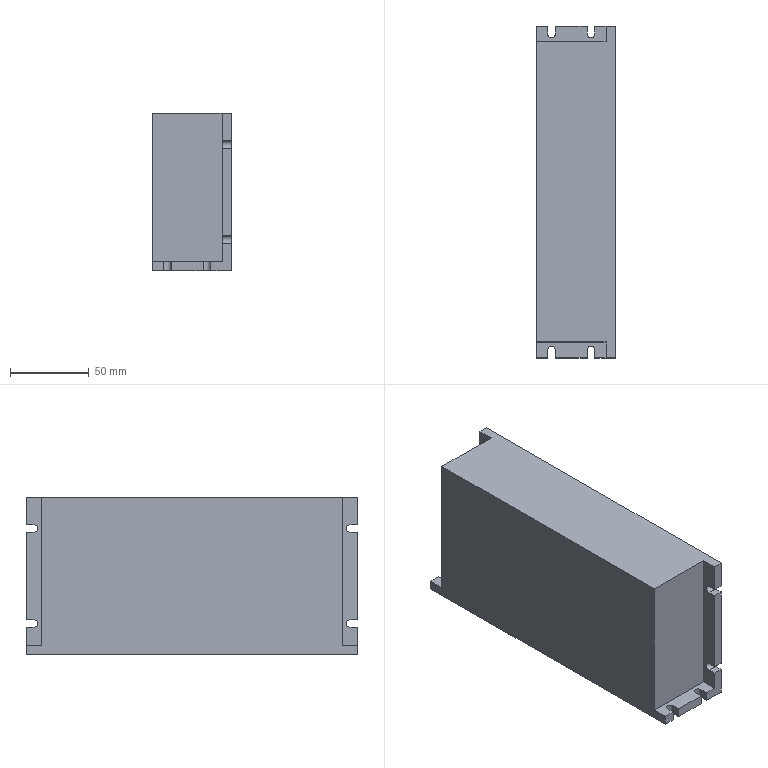Part | SolidWorks | features HoleWzd 2, Extrusion 1, ICE 1 | 1 solid | 44 faces | box 50 x 210 x 100 mm | volume 965694 mm3 | plane 36 | cylinder 8 | commonest cylinder face diameters 4.8 x8
STEP:
#1=CARTESIAN_POINT('',(-17.9,105.,6.));
#2=VERTEX_POINT('',#1);
#3=CARTESIAN_POINT('',(-25.,105.,6.));
#4=VERTEX_POINT('',#3);
#5=CARTESIAN_POINT('',(-25.,105.,6.));
#6=DIRECTION('',(-1.,0.,0.));
#7=VECTOR('',#6,1000.);
#8=LINE('',#5,#7);
#9=EDGE_CURVE('',#2,#4,#8,.T.);
#10=ORIENTED_EDGE('',*,*,#9,.F.);
#11=CARTESIAN_POINT('',(-17.9,105.,0.));
#12=VERTEX_POINT('',#11);
#13=CARTESIAN_POINT('',(-17.9,105.,100.));
#14=DIRECTION('',(0.,0.,-1.));
#15=VECTOR('',#14,1000.);
#16=LINE('',#13,#15);
#17=EDGE_CURVE('',#2,#12,#16,.T.);
#18=ORIENTED_EDGE('',*,*,#17,.T.);
#19=CARTESIAN_POINT('',(-25.,105.,0.));
#20=VERTEX_POINT('',#19);
#21=CARTESIAN_POINT('',(-25.,105.,0.));
#22=DIRECTION('',(-1.,0.,0.));
#23=VECTOR('',#22,1000.);
#24=LINE('',#21,#23);
#25=EDGE_CURVE('',#12,#20,#24,.T.);
#26=ORIENTED_EDGE('',*,*,#25,.T.);
#27=CARTESIAN_POINT('',(-25.,105.,100.));
#28=DIRECTION('',(0.,0.,-1.));
#29=VECTOR('',#28,1000.);
#30=LINE('',#27,#29);
#31=EDGE_CURVE('',#4,#20,#30,.T.);
#32=ORIENTED_EDGE('',*,*,#31,.F.);
#33=EDGE_LOOP('',(#10,#18,#26,#32));
#34=FACE_OUTER_BOUND('',#33,.T.);
#35=CARTESIAN_POINT('',(-25.,105.,100.));
#36=DIRECTION('',(0.,-1.,0.));
#37=DIRECTION('',(0.,0.,-1.));
#38=AXIS2_PLACEMENT_3D('',#35,#36,#37);
#39=PLANE('',#38);
#40=ADVANCED_FACE('',(#34),#39,.F.);
#41=CARTESIAN_POINT('',(7.1,105.,0.));
#42=VERTEX_POINT('',#41);
#43=CARTESIAN_POINT('',(-13.1,105.,0.));
#44=VERTEX_POINT('',#43);
#45=CARTESIAN_POINT('',(-25.,105.,0.));
#46=DIRECTION('',(-1.,0.,0.));
#47=VECTOR('',#46,1000.);
#48=LINE('',#45,#47);
#49=EDGE_CURVE('',#42,#44,#48,.T.);
#50=ORIENTED_EDGE('',*,*,#49,.T.);
#51=CARTESIAN_POINT('',(-13.1,105.,6.));
#52=VERTEX_POINT('',#51);
#53=CARTESIAN_POINT('',(-13.1,105.,100.));
#54=DIRECTION('',(0.,0.,1.));
#55=VECTOR('',#54,1000.);
#56=LINE('',#53,#55);
#57=EDGE_CURVE('',#44,#52,#56,.T.);
#58=ORIENTED_EDGE('',*,*,#57,.T.);
#59=CARTESIAN_POINT('',(7.1,105.,6.));
#60=VERTEX_POINT('',#59);
#61=CARTESIAN_POINT('',(-25.,105.,6.));
#62=DIRECTION('',(-1.,0.,0.));
#63=VECTOR('',#62,1000.);
#64=LINE('',#61,#63);
#65=EDGE_CURVE('',#60,#52,#64,.T.);
#66=ORIENTED_EDGE('',*,*,#65,.F.);
#67=CARTESIAN_POINT('',(7.1,105.,100.));
#68=DIRECTION('',(0.,0.,-1.));
#69=VECTOR('',#68,1000.);
#70=LINE('',#67,#69);
#71=EDGE_CURVE('',#60,#42,#70,.T.);
#72=ORIENTED_EDGE('',*,*,#71,.T.);
#73=EDGE_LOOP('',(#50,#58,#66,#72));
#74=FACE_OUTER_BOUND('',#73,.T.);
#75=CARTESIAN_POINT('',(-25.,105.,100.));
#76=DIRECTION('',(0.,-1.,0.));
#77=DIRECTION('',(0.,0.,-1.));
#78=AXIS2_PLACEMENT_3D('',#75,#76,#77);
#79=PLANE('',#78);
#80=ADVANCED_FACE('',(#74),#79,.F.);
#81=CARTESIAN_POINT('',(-13.1,-105.,0.));
#82=VERTEX_POINT('',#81);
#83=CARTESIAN_POINT('',(7.1,-105.,0.));
#84=VERTEX_POINT('',#83);
#85=CARTESIAN_POINT('',(-25.,-105.,0.));
#86=DIRECTION('',(1.,0.,0.));
#87=VECTOR('',#86,1000.);
#88=LINE('',#85,#87);
#89=EDGE_CURVE('',#82,#84,#88,.T.);
#90=ORIENTED_EDGE('',*,*,#89,.T.);
#91=CARTESIAN_POINT('',(7.1,-105.,6.));
#92=VERTEX_POINT('',#91);
#93=CARTESIAN_POINT('',(7.1,-105.,100.));
#94=DIRECTION('',(0.,0.,1.));
#95=VECTOR('',#94,1000.);
#96=LINE('',#93,#95);
#97=EDGE_CURVE('',#84,#92,#96,.T.);
#98=ORIENTED_EDGE('',*,*,#97,.T.);
#99=CARTESIAN_POINT('',(-13.1,-105.,6.));
#100=VERTEX_POINT('',#99);
#101=CARTESIAN_POINT('',(-25.,-105.,6.));
#102=DIRECTION('',(1.,0.,0.));
#103=VECTOR('',#102,1000.);
#104=LINE('',#101,#103);
#105=EDGE_CURVE('',#100,#92,#104,.T.);
#106=ORIENTED_EDGE('',*,*,#105,.F.);
#107=CARTESIAN_POINT('',(-13.1,-105.,100.));
#108=DIRECTION('',(0.,0.,-1.));
#109=VECTOR('',#108,1000.);
#110=LINE('',#107,#109);
#111=EDGE_CURVE('',#100,#82,#110,.T.);
#112=ORIENTED_EDGE('',*,*,#111,.T.);
#113=EDGE_LOOP('',(#90,#98,#106,#112));
#114=FACE_OUTER_BOUND('',#113,.T.);
#115=CARTESIAN_POINT('',(-25.,-105.,100.));
#116=DIRECTION('',(0.,1.,0.));
#117=DIRECTION('',(0.,0.,1.));
#118=AXIS2_PLACEMENT_3D('',#115,#116,#117);
#119=PLANE('',#118);
#120=ADVANCED_FACE('',(#114),#119,.F.);
#121=CARTESIAN_POINT('',(-25.,-105.,0.));
#122=VERTEX_POINT('',#121);
#123=CARTESIAN_POINT('',(-17.9,-105.,0.));
#124=VERTEX_POINT('',#123);
#125=CARTESIAN_POINT('',(-25.,-105.,0.));
#126=DIRECTION('',(1.,0.,0.));
#127=VECTOR('',#126,1000.);
#128=LINE('',#125,#127);
#129=EDGE_CURVE('',#122,#124,#128,.T.);
#130=ORIENTED_EDGE('',*,*,#129,.T.);
#131=CARTESIAN_POINT('',(-17.9,-105.,6.));
#132=VERTEX_POINT('',#131);
#133=CARTESIAN_POINT('',(-17.9,-105.,100.));
#134=DIRECTION('',(0.,0.,1.));
#135=VECTOR('',#134,1000.);
#136=LINE('',#133,#135);
#137=EDGE_CURVE('',#124,#132,#136,.T.);
#138=ORIENTED_EDGE('',*,*,#137,.T.);
#139=CARTESIAN_POINT('',(-25.,-105.,6.));
#140=VERTEX_POINT('',#139);
#141=CARTESIAN_POINT('',(-25.,-105.,6.));
#142=DIRECTION('',(1.,0.,0.));
#143=VECTOR('',#142,1000.);
#144=LINE('',#141,#143);
#145=EDGE_CURVE('',#140,#132,#144,.T.);
#146=ORIENTED_EDGE('',*,*,#145,.F.);
#147=CARTESIAN_POINT('',(-25.,-105.,100.));
#148=DIRECTION('',(0.,0.,-1.));
#149=VECTOR('',#148,1000.);
#150=LINE('',#147,#149);
#151=EDGE_CURVE('',#140,#122,#150,.T.);
#152=ORIENTED_EDGE('',*,*,#151,.T.);
#153=EDGE_LOOP('',(#130,#138,#146,#152));
#154=FACE_OUTER_BOUND('',#153,.T.);
#155=CARTESIAN_POINT('',(-25.,-105.,100.));
#156=DIRECTION('',(0.,1.,0.));
#157=DIRECTION('',(0.,0.,1.));
#158=AXIS2_PLACEMENT_3D('',#155,#156,#157);
#159=PLANE('',#158);
#160=ADVANCED_FACE('',(#154),#159,.F.);
#161=CARTESIAN_POINT('',(25.,105.,100.));
#162=VERTEX_POINT('',#161);
#163=CARTESIAN_POINT('',(25.,105.,82.4));
#164=VERTEX_POINT('',#163);
#165=CARTESIAN_POINT('',(25.,105.,100.));
#166=DIRECTION('',(0.,0.,-1.));
#167=VECTOR('',#166,1000.);
#168=LINE('',#165,#167);
#169=EDGE_CURVE('',#162,#164,#168,.T.);
#170=ORIENTED_EDGE('',*,*,#169,.T.);
#171=CARTESIAN_POINT('',(19.,105.,82.4));
#172=VERTEX_POINT('',#171);
#173=CARTESIAN_POINT('',(-25.,105.,82.4));
#174=DIRECTION('',(-1.,0.,0.));
#175=VECTOR('',#174,1000.);
#176=LINE('',#173,#175);
#177=EDGE_CURVE('',#164,#172,#176,.T.);
#178=ORIENTED_EDGE('',*,*,#177,.T.);
#179=CARTESIAN_POINT('',(19.,105.,100.));
#180=VERTEX_POINT('',#179);
#181=CARTESIAN_POINT('',(19.,105.,-45.122));
#182=DIRECTION('',(0.,0.,1.));
#183=VECTOR('',#182,1000.);
#184=LINE('',#181,#183);
#185=EDGE_CURVE('',#172,#180,#184,.T.);
#186=ORIENTED_EDGE('',*,*,#185,.T.);
#187=CARTESIAN_POINT('',(-25.,105.,100.));
#188=DIRECTION('',(-1.,0.,0.));
#189=VECTOR('',#188,1000.);
#190=LINE('',#187,#189);
#191=EDGE_CURVE('',#162,#180,#190,.T.);
#192=ORIENTED_EDGE('',*,*,#191,.F.);
#193=EDGE_LOOP('',(#170,#178,#186,#192));
#194=FACE_OUTER_BOUND('',#193,.T.);
#195=CARTESIAN_POINT('',(-25.,105.,100.));
#196=DIRECTION('',(0.,-1.,0.));
#197=DIRECTION('',(0.,0.,-1.));
#198=AXIS2_PLACEMENT_3D('',#195,#196,#197);
#199=PLANE('',#198);
#200=ADVANCED_FACE('',(#194),#199,.F.);
#201=CARTESIAN_POINT('',(19.,105.,22.4));
#202=VERTEX_POINT('',#201);
#203=CARTESIAN_POINT('',(19.,105.,77.6));
#204=VERTEX_POINT('',#203);
#205=CARTESIAN_POINT('',(19.,105.,-45.122));
#206=DIRECTION('',(0.,0.,1.));
#207=VECTOR('',#206,1000.);
#208=LINE('',#205,#207);
#209=EDGE_CURVE('',#202,#204,#208,.T.);
#210=ORIENTED_EDGE('',*,*,#209,.T.);
#211=CARTESIAN_POINT('',(25.,105.,77.6));
#212=VERTEX_POINT('',#211);
#213=CARTESIAN_POINT('',(-25.,105.,77.6));
#214=DIRECTION('',(1.,0.,0.));
#215=VECTOR('',#214,1000.);
#216=LINE('',#213,#215);
#217=EDGE_CURVE('',#204,#212,#216,.T.);
#218=ORIENTED_EDGE('',*,*,#217,.T.);
#219=CARTESIAN_POINT('',(25.,105.,22.4));
#220=VERTEX_POINT('',#219);
#221=CARTESIAN_POINT('',(25.,105.,100.));
#222=DIRECTION('',(0.,0.,-1.));
#223=VECTOR('',#222,1000.);
#224=LINE('',#221,#223);
#225=EDGE_CURVE('',#212,#220,#224,.T.);
#226=ORIENTED_EDGE('',*,*,#225,.T.);
#227=CARTESIAN_POINT('',(-25.,105.,22.4));
#228=DIRECTION('',(-1.,0.,0.));
#229=VECTOR('',#228,1000.);
#230=LINE('',#227,#229);
#231=EDGE_CURVE('',#220,#202,#230,.T.);
#232=ORIENTED_EDGE('',*,*,#231,.T.);
#233=EDGE_LOOP('',(#210,#218,#226,#232));
#234=FACE_OUTER_BOUND('',#233,.T.);
#235=CARTESIAN_POINT('',(-25.,105.,100.));
#236=DIRECTION('',(0.,-1.,0.));
#237=DIRECTION('',(0.,0.,-1.));
#238=AXIS2_PLACEMENT_3D('',#235,#236,#237);
#239=PLANE('',#238);
#240=ADVANCED_FACE('',(#234),#239,.F.);
#241=CARTESIAN_POINT('',(19.,-105.,22.4));
#242=VERTEX_POINT('',#241);
#243=CARTESIAN_POINT('',(19.,-105.,77.6));
#244=VERTEX_POINT('',#243);
#245=CARTESIAN_POINT('',(19.,-105.,-45.122));
#246=DIRECTION('',(0.,0.,1.));
#247=VECTOR('',#246,1000.);
#248=LINE('',#245,#247);
#249=EDGE_CURVE('',#242,#244,#248,.T.);
#250=ORIENTED_EDGE('',*,*,#249,.F.);
#251=CARTESIAN_POINT('',(25.,-105.,22.4));
#252=VERTEX_POINT('',#251);
#253=CARTESIAN_POINT('',(-25.,-105.,22.4));
#254=DIRECTION('',(1.,0.,0.));
#255=VECTOR('',#254,1000.);
#256=LINE('',#253,#255);
#257=EDGE_CURVE('',#242,#252,#256,.T.);
#258=ORIENTED_EDGE('',*,*,#257,.T.);
#259=CARTESIAN_POINT('',(25.,-105.,77.6));
#260=VERTEX_POINT('',#259);
#261=CARTESIAN_POINT('',(25.,-105.,100.));
#262=DIRECTION('',(0.,0.,-1.));
#263=VECTOR('',#262,1000.);
#264=LINE('',#261,#263);
#265=EDGE_CURVE('',#260,#252,#264,.T.);
#266=ORIENTED_EDGE('',*,*,#265,.F.);
#267=CARTESIAN_POINT('',(-25.,-105.,77.6));
#268=DIRECTION('',(-1.,0.,0.));
#269=VECTOR('',#268,1000.);
#270=LINE('',#267,#269);
#271=EDGE_CURVE('',#260,#244,#270,.T.);
#272=ORIENTED_EDGE('',*,*,#271,.T.);
#273=EDGE_LOOP('',(#250,#258,#266,#272));
#274=FACE_OUTER_BOUND('',#273,.T.);
#275=CARTESIAN_POINT('',(-25.,-105.,100.));
#276=DIRECTION('',(0.,1.,0.));
#277=DIRECTION('',(0.,0.,1.));
#278=AXIS2_PLACEMENT_3D('',#275,#276,#277);
#279=PLANE('',#278);
#280=ADVANCED_FACE('',(#274),#279,.F.);
#281=CARTESIAN_POINT('',(19.,-105.,82.4));
#282=VERTEX_POINT('',#281);
#283=CARTESIAN_POINT('',(19.,-105.,100.));
#284=VERTEX_POINT('',#283);
#285=CARTESIAN_POINT('',(19.,-105.,-45.122));
#286=DIRECTION('',(0.,0.,1.));
#287=VECTOR('',#286,1000.);
#288=LINE('',#285,#287);
#289=EDGE_CURVE('',#282,#284,#288,.T.);
#290=ORIENTED_EDGE('',*,*,#289,.F.);
#291=CARTESIAN_POINT('',(25.,-105.,82.4));
#292=VERTEX_POINT('',#291);
#293=CARTESIAN_POINT('',(-25.,-105.,82.4));
#294=DIRECTION('',(1.,0.,0.));
#295=VECTOR('',#294,1000.);
#296=LINE('',#293,#295);
#297=EDGE_CURVE('',#282,#292,#296,.T.);
#298=ORIENTED_EDGE('',*,*,#297,.T.);
#299=CARTESIAN_POINT('',(25.,-105.,100.));
#300=VERTEX_POINT('',#299);
#301=CARTESIAN_POINT('',(25.,-105.,100.));
#302=DIRECTION('',(0.,0.,-1.));
#303=VECTOR('',#302,1000.);
#304=LINE('',#301,#303);
#305=EDGE_CURVE('',#300,#292,#304,.T.);
#306=ORIENTED_EDGE('',*,*,#305,.F.);
#307=CARTESIAN_POINT('',(-25.,-105.,100.));
#308=DIRECTION('',(1.,0.,0.));
#309=VECTOR('',#308,1000.);
#310=LINE('',#307,#309);
#311=EDGE_CURVE('',#284,#300,#310,.T.);
#312=ORIENTED_EDGE('',*,*,#311,.F.);
#313=EDGE_LOOP('',(#290,#298,#306,#312));
#314=FACE_OUTER_BOUND('',#313,.T.);
#315=CARTESIAN_POINT('',(-25.,-105.,100.));
#316=DIRECTION('',(0.,1.,0.));
#317=DIRECTION('',(0.,0.,1.));
#318=AXIS2_PLACEMENT_3D('',#315,#316,#317);
#319=PLANE('',#318);
#320=ADVANCED_FACE('',(#314),#319,.F.);
#321=CARTESIAN_POINT('',(25.,100.,82.4));
#322=VERTEX_POINT('',#321);
#323=CARTESIAN_POINT('',(25.,100.,77.6));
#324=VERTEX_POINT('',#323);
#325=CARTESIAN_POINT('',(25.,100.,80.));
#326=DIRECTION('',(1.,0.,0.));
#327=DIRECTION('',(0.,0.,-1.));
#328=AXIS2_PLACEMENT_3D('',#325,#326,#327);
#329=CIRCLE('',#328,2.4);
#330=EDGE_CURVE('',#322,#324,#329,.T.);
#331=ORIENTED_EDGE('',*,*,#330,.F.);
#332=CARTESIAN_POINT('',(25.,100.,82.4));
#333=DIRECTION('',(0.,1.,0.));
#334=VECTOR('',#333,1000.);
#335=LINE('',#332,#334);
#336=EDGE_CURVE('',#322,#164,#335,.T.);
#337=ORIENTED_EDGE('',*,*,#336,.T.);
#338=ORIENTED_EDGE('',*,*,#169,.F.);
#339=CARTESIAN_POINT('',(25.,-105.,100.));
#340=DIRECTION('',(0.,1.,0.));
#341=VECTOR('',#340,1000.);
#342=LINE('',#339,#341);
#343=EDGE_CURVE('',#300,#162,#342,.T.);
#344=ORIENTED_EDGE('',*,*,#343,.F.);
#345=ORIENTED_EDGE('',*,*,#305,.T.);
#346=CARTESIAN_POINT('',(25.,-100.,82.4));
#347=VERTEX_POINT('',#346);
#348=CARTESIAN_POINT('',(25.,-110.,82.4));
#349=DIRECTION('',(0.,1.,0.));
#350=VECTOR('',#349,1000.);
#351=LINE('',#348,#350);
#352=EDGE_CURVE('',#292,#347,#351,.T.);
#353=ORIENTED_EDGE('',*,*,#352,.T.);
#354=CARTESIAN_POINT('',(25.,-100.,77.6));
#355=VERTEX_POINT('',#354);
#356=CARTESIAN_POINT('',(25.,-100.,80.));
#357=DIRECTION('',(1.,0.,0.));
#358=DIRECTION('',(0.,0.,-1.));
#359=AXIS2_PLACEMENT_3D('',#356,#357,#358);
#360=CIRCLE('',#359,2.4);
#361=EDGE_CURVE('',#355,#347,#360,.T.);
#362=ORIENTED_EDGE('',*,*,#361,.F.);
#363=CARTESIAN_POINT('',(25.,-110.,77.6));
#364=DIRECTION('',(0.,1.,0.));
#365=VECTOR('',#364,1000.);
#366=LINE('',#363,#365);
#367=EDGE_CURVE('',#260,#355,#366,.T.);
#368=ORIENTED_EDGE('',*,*,#367,.F.);
#369=ORIENTED_EDGE('',*,*,#265,.T.);
#370=CARTESIAN_POINT('',(25.,-100.,22.4));
#371=VERTEX_POINT('',#370);
#372=CARTESIAN_POINT('',(25.,-110.,22.4));
#373=DIRECTION('',(0.,1.,0.));
#374=VECTOR('',#373,1000.);
#375=LINE('',#372,#374);
#376=EDGE_CURVE('',#252,#371,#375,.T.);
#377=ORIENTED_EDGE('',*,*,#376,.T.);
#378=CARTESIAN_POINT('',(25.,-100.,17.6));
#379=VERTEX_POINT('',#378);
#380=CARTESIAN_POINT('',(25.,-100.,20.));
#381=DIRECTION('',(1.,0.,0.));
#382=DIRECTION('',(0.,0.,-1.));
#383=AXIS2_PLACEMENT_3D('',#380,#381,#382);
#384=CIRCLE('',#383,2.4);
#385=EDGE_CURVE('',#379,#371,#384,.T.);
#386=ORIENTED_EDGE('',*,*,#385,.F.);
#387=CARTESIAN_POINT('',(25.,-105.,17.6));
#388=VERTEX_POINT('',#387);
#389=CARTESIAN_POINT('',(25.,-110.,17.6));
#390=DIRECTION('',(0.,1.,0.));
#391=VECTOR('',#390,1000.);
#392=LINE('',#389,#391);
#393=EDGE_CURVE('',#388,#379,#392,.T.);
#394=ORIENTED_EDGE('',*,*,#393,.F.);
#395=CARTESIAN_POINT('',(25.,-105.,0.));
#396=VERTEX_POINT('',#395);
#397=CARTESIAN_POINT('',(25.,-105.,100.));
#398=DIRECTION('',(0.,0.,-1.));
#399=VECTOR('',#398,1000.);
#400=LINE('',#397,#399);
#401=EDGE_CURVE('',#388,#396,#400,.T.);
#402=ORIENTED_EDGE('',*,*,#401,.T.);
#403=CARTESIAN_POINT('',(25.,105.,0.));
#404=VERTEX_POINT('',#403);
#405=CARTESIAN_POINT('',(25.,-105.,0.));
#406=DIRECTION('',(0.,1.,0.));
#407=VECTOR('',#406,1000.);
#408=LINE('',#405,#407);
#409=EDGE_CURVE('',#396,#404,#408,.T.);
#410=ORIENTED_EDGE('',*,*,#409,.T.);
#411=CARTESIAN_POINT('',(25.,105.,17.6));
#412=VERTEX_POINT('',#411);
#413=CARTESIAN_POINT('',(25.,105.,100.));
#414=DIRECTION('',(0.,0.,-1.));
#415=VECTOR('',#414,1000.);
#416=LINE('',#413,#415);
#417=EDGE_CURVE('',#412,#404,#416,.T.);
#418=ORIENTED_EDGE('',*,*,#417,.F.);
#419=CARTESIAN_POINT('',(25.,100.,17.6));
#420=VERTEX_POINT('',#419);
#421=CARTESIAN_POINT('',(25.,100.,17.6));
#422=DIRECTION('',(0.,1.,0.));
#423=VECTOR('',#422,1000.);
#424=LINE('',#421,#423);
#425=EDGE_CURVE('',#420,#412,#424,.T.);
#426=ORIENTED_EDGE('',*,*,#425,.F.);
#427=CARTESIAN_POINT('',(25.,100.,22.4));
#428=VERTEX_POINT('',#427);
#429=CARTESIAN_POINT('',(25.,100.,20.));
#430=DIRECTION('',(1.,0.,0.));
#431=DIRECTION('',(0.,0.,-1.));
#432=AXIS2_PLACEMENT_3D('',#429,#430,#431);
#433=CIRCLE('',#432,2.4);
#434=EDGE_CURVE('',#428,#420,#433,.T.);
#435=ORIENTED_EDGE('',*,*,#434,.F.);
#436=CARTESIAN_POINT('',(25.,100.,22.4));
#437=DIRECTION('',(0.,1.,0.));
#438=VECTOR('',#437,1000.);
#439=LINE('',#436,#438);
#440=EDGE_CURVE('',#428,#220,#439,.T.);
#441=ORIENTED_EDGE('',*,*,#440,.T.);
#442=ORIENTED_EDGE('',*,*,#225,.F.);
#443=CARTESIAN_POINT('',(25.,100.,77.6));
#444=DIRECTION('',(0.,1.,0.));
#445=VECTOR('',#444,1000.);
#446=LINE('',#443,#445);
#447=EDGE_CURVE('',#324,#212,#446,.T.);
#448=ORIENTED_EDGE('',*,*,#447,.F.);
#449=EDGE_LOOP('',(#331,#337,#338,#344,#345,#353,#362,#368,#369,#377,#386,#394,#402,#410,#418,#426,#435,#441,#442,#448));
#450=FACE_OUTER_BOUND('',#449,.T.);
#451=CARTESIAN_POINT('',(25.,-105.,100.));
#452=DIRECTION('',(-1.,0.,0.));
#453=DIRECTION('',(0.,0.,1.));
#454=AXIS2_PLACEMENT_3D('',#451,#452,#453);
#455=PLANE('',#454);
#456=ADVANCED_FACE('',(#450),#455,.F.);
#457=CARTESIAN_POINT('',(11.9,105.,0.));
#458=VERTEX_POINT('',#457);
#459=CARTESIAN_POINT('',(-25.,105.,0.));
#460=DIRECTION('',(-1.,0.,0.));
#461=VECTOR('',#460,1000.);
#462=LINE('',#459,#461);
#463=EDGE_CURVE('',#404,#458,#462,.T.);
#464=ORIENTED_EDGE('',*,*,#463,.T.);
#465=CARTESIAN_POINT('',(11.9,105.,6.));
#466=VERTEX_POINT('',#465);
#467=CARTESIAN_POINT('',(11.9,105.,100.));
#468=DIRECTION('',(0.,0.,1.));
#469=VECTOR('',#468,1000.);
#470=LINE('',#467,#469);
#471=EDGE_CURVE('',#458,#466,#470,.T.);
#472=ORIENTED_EDGE('',*,*,#471,.T.);
#473=CARTESIAN_POINT('',(19.,105.,6.));
#474=VERTEX_POINT('',#473);
#475=CARTESIAN_POINT('',(-25.,105.,6.));
#476=DIRECTION('',(-1.,0.,0.));
#477=VECTOR('',#476,1000.);
#478=LINE('',#475,#477);
#479=EDGE_CURVE('',#474,#466,#478,.T.);
#480=ORIENTED_EDGE('',*,*,#479,.F.);
#481=CARTESIAN_POINT('',(19.,105.,17.6));
#482=VERTEX_POINT('',#481);
#483=CARTESIAN_POINT('',(19.,105.,-45.122));
#484=DIRECTION('',(0.,0.,1.));
#485=VECTOR('',#484,1000.);
#486=LINE('',#483,#485);
#487=EDGE_CURVE('',#474,#482,#486,.T.);
#488=ORIENTED_EDGE('',*,*,#487,.T.);
#489=CARTESIAN_POINT('',(-25.,105.,17.6));
#490=DIRECTION('',(1.,0.,0.));
#491=VECTOR('',#490,1000.);
#492=LINE('',#489,#491);
#493=EDGE_CURVE('',#482,#412,#492,.T.);
#494=ORIENTED_EDGE('',*,*,#493,.T.);
#495=ORIENTED_EDGE('',*,*,#417,.T.);
#496=EDGE_LOOP('',(#464,#472,#480,#488,#494,#495));
#497=FACE_OUTER_BOUND('',#496,.T.);
#498=CARTESIAN_POINT('',(-25.,105.,100.));
#499=DIRECTION('',(0.,-1.,0.));
#500=DIRECTION('',(0.,0.,-1.));
#501=AXIS2_PLACEMENT_3D('',#498,#499,#500);
#502=PLANE('',#501);
#503=ADVANCED_FACE('',(#497),#502,.F.);
#504=CARTESIAN_POINT('',(-25.,95.,6.));
#505=VERTEX_POINT('',#504);
#506=CARTESIAN_POINT('',(-25.,95.,100.));
#507=VERTEX_POINT('',#506);
#508=CARTESIAN_POINT('',(-25.,95.,-45.122));
#509=DIRECTION('',(0.,0.,1.));
#510=VECTOR('',#509,1000.);
#511=LINE('',#508,#510);
#512=EDGE_CURVE('',#505,#507,#511,.T.);
#513=ORIENTED_EDGE('',*,*,#512,.F.);
#514=CARTESIAN_POINT('',(-25.,105.,6.));
#515=DIRECTION('',(0.,-1.,0.));
#516=VECTOR('',#515,1000.);
#517=LINE('',#514,#516);
#518=EDGE_CURVE('',#4,#505,#517,.T.);
#519=ORIENTED_EDGE('',*,*,#518,.F.);
#520=ORIENTED_EDGE('',*,*,#31,.T.);
#521=CARTESIAN_POINT('',(-25.,-105.,0.));
#522=DIRECTION('',(0.,-1.,0.));
#523=VECTOR('',#522,1000.);
#524=LINE('',#521,#523);
#525=EDGE_CURVE('',#20,#122,#524,.T.);
#526=ORIENTED_EDGE('',*,*,#525,.T.);
#527=ORIENTED_EDGE('',*,*,#151,.F.);
#528=CARTESIAN_POINT('',(-25.,-95.,6.));
#529=VERTEX_POINT('',#528);
#530=CARTESIAN_POINT('',(-25.,-105.,6.));
#531=DIRECTION('',(0.,-1.,0.));
#532=VECTOR('',#531,1000.);
#533=LINE('',#530,#532);
#534=EDGE_CURVE('',#529,#140,#533,.T.);
#535=ORIENTED_EDGE('',*,*,#534,.F.);
#536=CARTESIAN_POINT('',(-25.,-95.,100.));
#537=VERTEX_POINT('',#536);
#538=CARTESIAN_POINT('',(-25.,-95.,-45.122));
#539=DIRECTION('',(0.,0.,1.));
#540=VECTOR('',#539,1000.);
#541=LINE('',#538,#540);
#542=EDGE_CURVE('',#529,#537,#541,.T.);
#543=ORIENTED_EDGE('',*,*,#542,.T.);
#544=CARTESIAN_POINT('',(-25.,-105.,100.));
#545=DIRECTION('',(0.,-1.,0.));
#546=VECTOR('',#545,1000.);
#547=LINE('',#544,#546);
#548=EDGE_CURVE('',#507,#537,#547,.T.);
#549=ORIENTED_EDGE('',*,*,#548,.F.);
#550=EDGE_LOOP('',(#513,#519,#520,#526,#527,#535,#543,#549));
#551=FACE_OUTER_BOUND('',#550,.T.);
#552=CARTESIAN_POINT('',(-25.,-105.,100.));
#553=DIRECTION('',(1.,0.,0.));
#554=DIRECTION('',(0.,0.,-1.));
#555=AXIS2_PLACEMENT_3D('',#552,#553,#554);
#556=PLANE('',#555);
#557=ADVANCED_FACE('',(#551),#556,.F.);
#558=CARTESIAN_POINT('',(11.9,-105.,6.));
#559=VERTEX_POINT('',#558);
#560=CARTESIAN_POINT('',(19.,-105.,6.));
#561=VERTEX_POINT('',#560);
#562=CARTESIAN_POINT('',(-25.,-105.,6.));
#563=DIRECTION('',(1.,0.,0.));
#564=VECTOR('',#563,1000.);
#565=LINE('',#562,#564);
#566=EDGE_CURVE('',#559,#561,#565,.T.);
#567=ORIENTED_EDGE('',*,*,#566,.F.);
#568=CARTESIAN_POINT('',(11.9,-105.,0.));
#569=VERTEX_POINT('',#568);
#570=CARTESIAN_POINT('',(11.9,-105.,100.));
#571=DIRECTION('',(0.,0.,-1.));
#572=VECTOR('',#571,1000.);
#573=LINE('',#570,#572);
#574=EDGE_CURVE('',#559,#569,#573,.T.);
#575=ORIENTED_EDGE('',*,*,#574,.T.);
#576=CARTESIAN_POINT('',(-25.,-105.,0.));
#577=DIRECTION('',(1.,0.,0.));
#578=VECTOR('',#577,1000.);
#579=LINE('',#576,#578);
#580=EDGE_CURVE('',#569,#396,#579,.T.);
#581=ORIENTED_EDGE('',*,*,#580,.T.);
#582=ORIENTED_EDGE('',*,*,#401,.F.);
#583=CARTESIAN_POINT('',(19.,-105.,17.6));
#584=VERTEX_POINT('',#583);
#585=CARTESIAN_POINT('',(-25.,-105.,17.6));
#586=DIRECTION('',(-1.,0.,0.));
#587=VECTOR('',#586,1000.);
#588=LINE('',#585,#587);
#589=EDGE_CURVE('',#388,#584,#588,.T.);
#590=ORIENTED_EDGE('',*,*,#589,.T.);
#591=CARTESIAN_POINT('',(19.,-105.,-45.122));
#592=DIRECTION('',(0.,0.,1.));
#593=VECTOR('',#592,1000.);
#594=LINE('',#591,#593);
#595=EDGE_CURVE('',#561,#584,#594,.T.);
#596=ORIENTED_EDGE('',*,*,#595,.F.);
#597=EDGE_LOOP('',(#567,#575,#581,#582,#590,#596));
#598=FACE_OUTER_BOUND('',#597,.T.);
#599=CARTESIAN_POINT('',(-25.,-105.,100.));
#600=DIRECTION('',(0.,1.,0.));
#601=DIRECTION('',(0.,0.,1.));
#602=AXIS2_PLACEMENT_3D('',#599,#600,#601);
#603=PLANE('',#602);
#604=ADVANCED_FACE('',(#598),#603,.F.);
#605=CARTESIAN_POINT('',(19.,95.,100.));
#606=VERTEX_POINT('',#605);
#607=CARTESIAN_POINT('',(19.,105.,100.));
#608=DIRECTION('',(0.,1.,0.));
#609=VECTOR('',#608,1000.);
#610=LINE('',#607,#609);
#611=EDGE_CURVE('',#606,#180,#610,.T.);
#612=ORIENTED_EDGE('',*,*,#611,.F.);
#613=CARTESIAN_POINT('',(-25.,95.,100.));
#614=DIRECTION('',(1.,0.,0.));
#615=VECTOR('',#614,1000.);
#616=LINE('',#613,#615);
#617=EDGE_CURVE('',#507,#606,#616,.T.);
#618=ORIENTED_EDGE('',*,*,#617,.F.);
#619=ORIENTED_EDGE('',*,*,#548,.T.);
#620=CARTESIAN_POINT('',(19.,-95.,100.));
#621=VERTEX_POINT('',#620);
#622=CARTESIAN_POINT('',(-25.,-95.,100.));
#623=DIRECTION('',(-1.,0.,0.));
#624=VECTOR('',#623,1000.);
#625=LINE('',#622,#624);
#626=EDGE_CURVE('',#621,#537,#625,.T.);
#627=ORIENTED_EDGE('',*,*,#626,.F.);
#628=CARTESIAN_POINT('',(19.,-105.,100.));
#629=DIRECTION('',(0.,1.,0.));
#630=VECTOR('',#629,1000.);
#631=LINE('',#628,#630);
#632=EDGE_CURVE('',#284,#621,#631,.T.);
#633=ORIENTED_EDGE('',*,*,#632,.F.);
#634=ORIENTED_EDGE('',*,*,#311,.T.);
#635=ORIENTED_EDGE('',*,*,#343,.T.);
#636=ORIENTED_EDGE('',*,*,#191,.T.);
#637=EDGE_LOOP('',(#612,#618,#619,#627,#633,#634,#635,#636));
#638=FACE_OUTER_BOUND('',#637,.T.);
#639=CARTESIAN_POINT('',(0.,0.,100.));
#640=DIRECTION('',(0.,0.,-1.));
#641=DIRECTION('',(-1.,0.,0.));
#642=AXIS2_PLACEMENT_3D('',#639,#640,#641);
#643=PLANE('',#642);
#644=ADVANCED_FACE('',(#638),#643,.F.);
#645=CARTESIAN_POINT('',(-17.9,100.,0.));
#646=VERTEX_POINT('',#645);
#647=CARTESIAN_POINT('',(-17.9,100.,0.));
#648=DIRECTION('',(0.,1.,0.));
#649=VECTOR('',#648,1000.);
#650=LINE('',#647,#649);
#651=EDGE_CURVE('',#646,#12,#650,.T.);
#652=ORIENTED_EDGE('',*,*,#651,.F.);
#653=CARTESIAN_POINT('',(-13.1,100.,0.));
#654=VERTEX_POINT('',#653);
#655=CARTESIAN_POINT('',(-15.5,100.,0.));
#656=DIRECTION('',(0.,0.,1.));
#657=DIRECTION('',(1.,0.,0.));
#658=AXIS2_PLACEMENT_3D('',#655,#656,#657);
#659=CIRCLE('',#658,2.4);
#660=EDGE_CURVE('',#646,#654,#659,.T.);
#661=ORIENTED_EDGE('',*,*,#660,.T.);
#662=CARTESIAN_POINT('',(-13.1,100.,0.));
#663=DIRECTION('',(0.,1.,0.));
#664=VECTOR('',#663,1000.);
#665=LINE('',#662,#664);
#666=EDGE_CURVE('',#654,#44,#665,.T.);
#667=ORIENTED_EDGE('',*,*,#666,.T.);
#668=ORIENTED_EDGE('',*,*,#49,.F.);
#669=CARTESIAN_POINT('',(7.1,100.,0.));
#670=VERTEX_POINT('',#669);
#671=CARTESIAN_POINT('',(7.1,100.,0.));
#672=DIRECTION('',(0.,1.,0.));
#673=VECTOR('',#672,1000.);
#674=LINE('',#671,#673);
#675=EDGE_CURVE('',#670,#42,#674,.T.);
#676=ORIENTED_EDGE('',*,*,#675,.F.);
#677=CARTESIAN_POINT('',(11.9,100.,0.));
#678=VERTEX_POINT('',#677);
#679=CARTESIAN_POINT('',(9.5,100.,0.));
#680=DIRECTION('',(0.,0.,1.));
#681=DIRECTION('',(1.,0.,0.));
#682=AXIS2_PLACEMENT_3D('',#679,#680,#681);
#683=CIRCLE('',#682,2.4);
#684=EDGE_CURVE('',#670,#678,#683,.T.);
#685=ORIENTED_EDGE('',*,*,#684,.T.);
#686=CARTESIAN_POINT('',(11.9,100.,0.));
#687=DIRECTION('',(0.,1.,0.));
#688=VECTOR('',#687,1000.);
#689=LINE('',#686,#688);
#690=EDGE_CURVE('',#678,#458,#689,.T.);
#691=ORIENTED_EDGE('',*,*,#690,.T.);
#692=ORIENTED_EDGE('',*,*,#463,.F.);
#693=ORIENTED_EDGE('',*,*,#409,.F.);
#694=ORIENTED_EDGE('',*,*,#580,.F.);
#695=CARTESIAN_POINT('',(11.9,-100.,0.));
#696=VERTEX_POINT('',#695);
#697=CARTESIAN_POINT('',(11.9,0.,0.));
#698=DIRECTION('',(0.,-1.,0.));
#699=VECTOR('',#698,1000.);
#700=LINE('',#697,#699);
#701=EDGE_CURVE('',#696,#569,#700,.T.);
#702=ORIENTED_EDGE('',*,*,#701,.F.);
#703=CARTESIAN_POINT('',(7.1,-100.,0.));
#704=VERTEX_POINT('',#703);
#705=CARTESIAN_POINT('',(9.5,-100.,0.));
#706=DIRECTION('',(0.,0.,1.));
#707=DIRECTION('',(1.,0.,0.));
#708=AXIS2_PLACEMENT_3D('',#705,#706,#707);
#709=CIRCLE('',#708,2.4);
#710=EDGE_CURVE('',#696,#704,#709,.T.);
#711=ORIENTED_EDGE('',*,*,#710,.T.);
#712=CARTESIAN_POINT('',(7.1,0.,0.));
#713=DIRECTION('',(0.,1.,0.));
#714=VECTOR('',#713,1000.);
#715=LINE('',#712,#714);
#716=EDGE_CURVE('',#84,#704,#715,.T.);
#717=ORIENTED_EDGE('',*,*,#716,.F.);
#718=ORIENTED_EDGE('',*,*,#89,.F.);
#719=CARTESIAN_POINT('',(-13.1,-100.,0.));
#720=VERTEX_POINT('',#719);
#721=CARTESIAN_POINT('',(-13.1,-110.,0.));
#722=DIRECTION('',(0.,1.,0.));
#723=VECTOR('',#722,1000.);
#724=LINE('',#721,#723);
#725=EDGE_CURVE('',#82,#720,#724,.T.);
#726=ORIENTED_EDGE('',*,*,#725,.T.);
#727=CARTESIAN_POINT('',(-17.9,-100.,0.));
#728=VERTEX_POINT('',#727);
#729=CARTESIAN_POINT('',(-15.5,-100.,0.));
#730=DIRECTION('',(0.,0.,1.));
#731=DIRECTION('',(1.,0.,0.));
#732=AXIS2_PLACEMENT_3D('',#729,#730,#731);
#733=CIRCLE('',#732,2.4);
#734=EDGE_CURVE('',#720,#728,#733,.T.);
#735=ORIENTED_EDGE('',*,*,#734,.T.);
#736=CARTESIAN_POINT('',(-17.9,-110.,0.));
#737=DIRECTION('',(0.,1.,0.));
#738=VECTOR('',#737,1000.);
#739=LINE('',#736,#738);
#740=EDGE_CURVE('',#124,#728,#739,.T.);
#741=ORIENTED_EDGE('',*,*,#740,.F.);
#742=ORIENTED_EDGE('',*,*,#129,.F.);
#743=ORIENTED_EDGE('',*,*,#525,.F.);
#744=ORIENTED_EDGE('',*,*,#25,.F.);
#745=EDGE_LOOP('',(#652,#661,#667,#668,#676,#685,#691,#692,#693,#694,#702,#711,#717,#718,#726,#735,#741,#742,#743,#744));
#746=FACE_OUTER_BOUND('',#745,.T.);
#747=CARTESIAN_POINT('',(0.,0.,0.));
#748=DIRECTION('',(0.,0.,-1.));
#749=DIRECTION('',(-1.,0.,0.));
#750=AXIS2_PLACEMENT_3D('',#747,#748,#749);
#751=PLANE('',#750);
#752=ADVANCED_FACE('',(#746),#751,.T.);
#753=CARTESIAN_POINT('',(11.9,-100.,6.));
#754=VERTEX_POINT('',#753);
#755=CARTESIAN_POINT('',(7.1,-100.,6.));
#756=VERTEX_POINT('',#755);
#757=CARTESIAN_POINT('',(9.5,-100.,6.));
#758=DIRECTION('',(0.,0.,1.));
#759=DIRECTION('',(1.,0.,0.));
#760=AXIS2_PLACEMENT_3D('',#757,#758,#759);
#761=CIRCLE('',#760,2.4);
#762=EDGE_CURVE('',#754,#756,#761,.T.);
#763=ORIENTED_EDGE('',*,*,#762,.F.);
#764=CARTESIAN_POINT('',(11.9,-110.,6.));
#765=DIRECTION('',(0.,1.,0.));
#766=VECTOR('',#765,1000.);
#767=LINE('',#764,#766);
#768=EDGE_CURVE('',#559,#754,#767,.T.);
#769=ORIENTED_EDGE('',*,*,#768,.F.);
#770=ORIENTED_EDGE('',*,*,#566,.T.);
#771=CARTESIAN_POINT('',(19.,-95.,6.));
#772=VERTEX_POINT('',#771);
#773=CARTESIAN_POINT('',(19.,-105.,6.));
#774=DIRECTION('',(0.,1.,0.));
#775=VECTOR('',#774,1000.);
#776=LINE('',#773,#775);
#777=EDGE_CURVE('',#561,#772,#776,.T.);
#778=ORIENTED_EDGE('',*,*,#777,.T.);
#779=CARTESIAN_POINT('',(-25.,-95.,6.));
#780=DIRECTION('',(-1.,0.,0.));
#781=VECTOR('',#780,1000.);
#782=LINE('',#779,#781);
#783=EDGE_CURVE('',#772,#529,#782,.T.);
#784=ORIENTED_EDGE('',*,*,#783,.T.);
#785=ORIENTED_EDGE('',*,*,#534,.T.);
#786=ORIENTED_EDGE('',*,*,#145,.T.);
#787=CARTESIAN_POINT('',(-17.9,-100.,6.));
#788=VERTEX_POINT('',#787);
#789=CARTESIAN_POINT('',(-17.9,-110.,6.));
#790=DIRECTION('',(0.,1.,0.));
#791=VECTOR('',#790,1000.);
#792=LINE('',#789,#791);
#793=EDGE_CURVE('',#132,#788,#792,.T.);
#794=ORIENTED_EDGE('',*,*,#793,.T.);
#795=CARTESIAN_POINT('',(-13.1,-100.,6.));
#796=VERTEX_POINT('',#795);
#797=CARTESIAN_POINT('',(-15.5,-100.,6.));
#798=DIRECTION('',(0.,0.,1.));
#799=DIRECTION('',(1.,0.,0.));
#800=AXIS2_PLACEMENT_3D('',#797,#798,#799);
#801=CIRCLE('',#800,2.4);
#802=EDGE_CURVE('',#796,#788,#801,.T.);
#803=ORIENTED_EDGE('',*,*,#802,.F.);
#804=CARTESIAN_POINT('',(-13.1,0.,6.));
#805=DIRECTION('',(0.,-1.,0.));
#806=VECTOR('',#805,1000.);
#807=LINE('',#804,#806);
#808=EDGE_CURVE('',#796,#100,#807,.T.);
#809=ORIENTED_EDGE('',*,*,#808,.T.);
#810=ORIENTED_EDGE('',*,*,#105,.T.);
#811=CARTESIAN_POINT('',(7.1,0.,6.));
#812=DIRECTION('',(0.,1.,0.));
#813=VECTOR('',#812,1000.);
#814=LINE('',#811,#813);
#815=EDGE_CURVE('',#92,#756,#814,.T.);
#816=ORIENTED_EDGE('',*,*,#815,.T.);
#817=EDGE_LOOP('',(#763,#769,#770,#778,#784,#785,#786,#794,#803,#809,#810,#816));
#818=FACE_OUTER_BOUND('',#817,.T.);
#819=CARTESIAN_POINT('',(0.,0.,6.));
#820=DIRECTION('',(0.,0.,-1.));
#821=DIRECTION('',(-1.,0.,0.));
#822=AXIS2_PLACEMENT_3D('',#819,#820,#821);
#823=PLANE('',#822);
#824=ADVANCED_FACE('',(#818),#823,.F.);
#825=CARTESIAN_POINT('',(19.,-100.,17.6));
#826=VERTEX_POINT('',#825);
#827=CARTESIAN_POINT('',(19.,-100.,22.4));
#828=VERTEX_POINT('',#827);
#829=CARTESIAN_POINT('',(19.,-100.,20.));
#830=DIRECTION('',(1.,0.,0.));
#831=DIRECTION('',(0.,1.,0.));
#832=AXIS2_PLACEMENT_3D('',#829,#830,#831);
#833=CIRCLE('',#832,2.4);
#834=EDGE_CURVE('',#826,#828,#833,.T.);
#835=ORIENTED_EDGE('',*,*,#834,.T.);
#836=CARTESIAN_POINT('',(19.,-105.,22.4));
#837=DIRECTION('',(0.,-1.,0.));
#838=VECTOR('',#837,1000.);
#839=LINE('',#836,#838);
#840=EDGE_CURVE('',#828,#242,#839,.T.);
#841=ORIENTED_EDGE('',*,*,#840,.T.);
#842=ORIENTED_EDGE('',*,*,#249,.T.);
#843=CARTESIAN_POINT('',(19.,-100.,77.6));
#844=VERTEX_POINT('',#843);
#845=CARTESIAN_POINT('',(19.,-105.,77.6));
#846=DIRECTION('',(0.,1.,0.));
#847=VECTOR('',#846,1000.);
#848=LINE('',#845,#847);
#849=EDGE_CURVE('',#244,#844,#848,.T.);
#850=ORIENTED_EDGE('',*,*,#849,.T.);
#851=CARTESIAN_POINT('',(19.,-100.,82.4));
#852=VERTEX_POINT('',#851);
#853=CARTESIAN_POINT('',(19.,-100.,80.));
#854=DIRECTION('',(1.,0.,0.));
#855=DIRECTION('',(0.,1.,0.));
#856=AXIS2_PLACEMENT_3D('',#853,#854,#855);
#857=CIRCLE('',#856,2.4);
#858=EDGE_CURVE('',#844,#852,#857,.T.);
#859=ORIENTED_EDGE('',*,*,#858,.T.);
#860=CARTESIAN_POINT('',(19.,-105.,82.4));
#861=DIRECTION('',(0.,-1.,0.));
#862=VECTOR('',#861,1000.);
#863=LINE('',#860,#862);
#864=EDGE_CURVE('',#852,#282,#863,.T.);
#865=ORIENTED_EDGE('',*,*,#864,.T.);
#866=ORIENTED_EDGE('',*,*,#289,.T.);
#867=ORIENTED_EDGE('',*,*,#632,.T.);
#868=CARTESIAN_POINT('',(19.,-95.,-45.122));
#869=DIRECTION('',(0.,0.,1.));
#870=VECTOR('',#869,1000.);
#871=LINE('',#868,#870);
#872=EDGE_CURVE('',#772,#621,#871,.T.);
#873=ORIENTED_EDGE('',*,*,#872,.F.);
#874=ORIENTED_EDGE('',*,*,#777,.F.);
#875=ORIENTED_EDGE('',*,*,#595,.T.);
#876=CARTESIAN_POINT('',(19.,-105.,17.6));
#877=DIRECTION('',(0.,1.,0.));
#878=VECTOR('',#877,1000.);
#879=LINE('',#876,#878);
#880=EDGE_CURVE('',#584,#826,#879,.T.);
#881=ORIENTED_EDGE('',*,*,#880,.T.);
#882=EDGE_LOOP('',(#835,#841,#842,#850,#859,#865,#866,#867,#873,#874,#875,#881));
#883=FACE_OUTER_BOUND('',#882,.T.);
#884=CARTESIAN_POINT('',(19.,-105.,-45.122));
#885=DIRECTION('',(1.,0.,0.));
#886=DIRECTION('',(0.,1.,0.));
#887=AXIS2_PLACEMENT_3D('',#884,#885,#886);
#888=PLANE('',#887);
#889=ADVANCED_FACE('',(#883),#888,.F.);
#890=ORIENTED_EDGE('',*,*,#872,.T.);
#891=ORIENTED_EDGE('',*,*,#626,.T.);
#892=ORIENTED_EDGE('',*,*,#542,.F.);
#893=ORIENTED_EDGE('',*,*,#783,.F.);
#894=EDGE_LOOP('',(#890,#891,#892,#893));
#895=FACE_OUTER_BOUND('',#894,.T.);
#896=CARTESIAN_POINT('',(-25.,-95.,-45.122));
#897=DIRECTION('',(0.,1.,0.));
#898=DIRECTION('',(-1.,0.,0.));
#899=AXIS2_PLACEMENT_3D('',#896,#897,#898);
#900=PLANE('',#899);
#901=ADVANCED_FACE('',(#895),#900,.F.);
#902=CARTESIAN_POINT('',(-17.9,100.,6.));
#903=VERTEX_POINT('',#902);
#904=CARTESIAN_POINT('',(-13.1,100.,6.));
#905=VERTEX_POINT('',#904);
#906=CARTESIAN_POINT('',(-15.5,100.,6.));
#907=DIRECTION('',(0.,0.,1.));
#908=DIRECTION('',(1.,0.,0.));
#909=AXIS2_PLACEMENT_3D('',#906,#907,#908);
#910=CIRCLE('',#909,2.4);
#911=EDGE_CURVE('',#903,#905,#910,.T.);
#912=ORIENTED_EDGE('',*,*,#911,.F.);
#913=CARTESIAN_POINT('',(-17.9,100.,6.));
#914=DIRECTION('',(0.,1.,0.));
#915=VECTOR('',#914,1000.);
#916=LINE('',#913,#915);
#917=EDGE_CURVE('',#903,#2,#916,.T.);
#918=ORIENTED_EDGE('',*,*,#917,.T.);
#919=ORIENTED_EDGE('',*,*,#9,.T.);
#920=ORIENTED_EDGE('',*,*,#518,.T.);
#921=CARTESIAN_POINT('',(19.,95.,6.));
#922=VERTEX_POINT('',#921);
#923=CARTESIAN_POINT('',(-25.,95.,6.));
#924=DIRECTION('',(1.,0.,0.));
#925=VECTOR('',#924,1000.);
#926=LINE('',#923,#925);
#927=EDGE_CURVE('',#505,#922,#926,.T.);
#928=ORIENTED_EDGE('',*,*,#927,.T.);
#929=CARTESIAN_POINT('',(19.,105.,6.));
#930=DIRECTION('',(0.,1.,0.));
#931=VECTOR('',#930,1000.);
#932=LINE('',#929,#931);
#933=EDGE_CURVE('',#922,#474,#932,.T.);
#934=ORIENTED_EDGE('',*,*,#933,.T.);
#935=ORIENTED_EDGE('',*,*,#479,.T.);
#936=CARTESIAN_POINT('',(11.9,100.,6.));
#937=VERTEX_POINT('',#936);
#938=CARTESIAN_POINT('',(11.9,100.,6.));
#939=DIRECTION('',(0.,1.,0.));
#940=VECTOR('',#939,1000.);
#941=LINE('',#938,#940);
#942=EDGE_CURVE('',#937,#466,#941,.T.);
#943=ORIENTED_EDGE('',*,*,#942,.F.);
#944=CARTESIAN_POINT('',(7.1,100.,6.));
#945=VERTEX_POINT('',#944);
#946=CARTESIAN_POINT('',(9.5,100.,6.));
#947=DIRECTION('',(0.,0.,1.));
#948=DIRECTION('',(1.,0.,0.));
#949=AXIS2_PLACEMENT_3D('',#946,#947,#948);
#950=CIRCLE('',#949,2.4);
#951=EDGE_CURVE('',#945,#937,#950,.T.);
#952=ORIENTED_EDGE('',*,*,#951,.F.);
#953=CARTESIAN_POINT('',(7.1,100.,6.));
#954=DIRECTION('',(0.,1.,0.));
#955=VECTOR('',#954,1000.);
#956=LINE('',#953,#955);
#957=EDGE_CURVE('',#945,#60,#956,.T.);
#958=ORIENTED_EDGE('',*,*,#957,.T.);
#959=ORIENTED_EDGE('',*,*,#65,.T.);
#960=CARTESIAN_POINT('',(-13.1,100.,6.));
#961=DIRECTION('',(0.,1.,0.));
#962=VECTOR('',#961,1000.);
#963=LINE('',#960,#962);
#964=EDGE_CURVE('',#905,#52,#963,.T.);
#965=ORIENTED_EDGE('',*,*,#964,.F.);
#966=EDGE_LOOP('',(#912,#918,#919,#920,#928,#934,#935,#943,#952,#958,#959,#965));
#967=FACE_OUTER_BOUND('',#966,.T.);
#968=CARTESIAN_POINT('',(0.,0.,6.));
#969=DIRECTION('',(0.,0.,-1.));
#970=DIRECTION('',(-1.,0.,0.));
#971=AXIS2_PLACEMENT_3D('',#968,#969,#970);
#972=PLANE('',#971);
#973=ADVANCED_FACE('',(#967),#972,.F.);
#974=ORIENTED_EDGE('',*,*,#512,.T.);
#975=ORIENTED_EDGE('',*,*,#617,.T.);
#976=CARTESIAN_POINT('',(19.,95.,-45.122));
#977=DIRECTION('',(0.,0.,1.));
#978=VECTOR('',#977,1000.);
#979=LINE('',#976,#978);
#980=EDGE_CURVE('',#922,#606,#979,.T.);
#981=ORIENTED_EDGE('',*,*,#980,.F.);
#982=ORIENTED_EDGE('',*,*,#927,.F.);
#983=EDGE_LOOP('',(#974,#975,#981,#982));
#984=FACE_OUTER_BOUND('',#983,.T.);
#985=CARTESIAN_POINT('',(-25.,95.,-45.122));
#986=DIRECTION('',(0.,-1.,0.));
#987=DIRECTION('',(1.,0.,0.));
#988=AXIS2_PLACEMENT_3D('',#985,#986,#987);
#989=PLANE('',#988);
#990=ADVANCED_FACE('',(#984),#989,.F.);
#991=CARTESIAN_POINT('',(19.,100.,82.4));
#992=VERTEX_POINT('',#991);
#993=CARTESIAN_POINT('',(19.,100.,77.6));
#994=VERTEX_POINT('',#993);
#995=CARTESIAN_POINT('',(19.,100.,80.));
#996=DIRECTION('',(1.,0.,0.));
#997=DIRECTION('',(0.,1.,0.));
#998=AXIS2_PLACEMENT_3D('',#995,#996,#997);
#999=CIRCLE('',#998,2.4);
#1000=EDGE_CURVE('',#992,#994,#999,.T.);
#1001=ORIENTED_EDGE('',*,*,#1000,.T.);
#1002=CARTESIAN_POINT('',(19.,105.,77.6));
#1003=DIRECTION('',(0.,1.,0.));
#1004=VECTOR('',#1003,1000.);
#1005=LINE('',#1002,#1004);
#1006=EDGE_CURVE('',#994,#204,#1005,.T.);
#1007=ORIENTED_EDGE('',*,*,#1006,.T.);
#1008=ORIENTED_EDGE('',*,*,#209,.F.);
#1009=CARTESIAN_POINT('',(19.,100.,22.4));
#1010=VERTEX_POINT('',#1009);
#1011=CARTESIAN_POINT('',(19.,105.,22.4));
#1012=DIRECTION('',(0.,-1.,0.));
#1013=VECTOR('',#1012,1000.);
#1014=LINE('',#1011,#1013);
#1015=EDGE_CURVE('',#202,#1010,#1014,.T.);
#1016=ORIENTED_EDGE('',*,*,#1015,.T.);
#1017=CARTESIAN_POINT('',(19.,100.,17.6));
#1018=VERTEX_POINT('',#1017);
#1019=CARTESIAN_POINT('',(19.,100.,20.));
#1020=DIRECTION('',(1.,0.,0.));
#1021=DIRECTION('',(0.,1.,0.));
#1022=AXIS2_PLACEMENT_3D('',#1019,#1020,#1021);
#1023=CIRCLE('',#1022,2.4);
#1024=EDGE_CURVE('',#1010,#1018,#1023,.T.);
#1025=ORIENTED_EDGE('',*,*,#1024,.T.);
#1026=CARTESIAN_POINT('',(19.,105.,17.6));
#1027=DIRECTION('',(0.,1.,0.));
#1028=VECTOR('',#1027,1000.);
#1029=LINE('',#1026,#1028);
#1030=EDGE_CURVE('',#1018,#482,#1029,.T.);
#1031=ORIENTED_EDGE('',*,*,#1030,.T.);
#1032=ORIENTED_EDGE('',*,*,#487,.F.);
#1033=ORIENTED_EDGE('',*,*,#933,.F.);
#1034=ORIENTED_EDGE('',*,*,#980,.T.);
#1035=ORIENTED_EDGE('',*,*,#611,.T.);
#1036=ORIENTED_EDGE('',*,*,#185,.F.);
#1037=CARTESIAN_POINT('',(19.,105.,82.4));
#1038=DIRECTION('',(0.,-1.,0.));
#1039=VECTOR('',#1038,1000.);
#1040=LINE('',#1037,#1039);
#1041=EDGE_CURVE('',#172,#992,#1040,.T.);
#1042=ORIENTED_EDGE('',*,*,#1041,.T.);
#1043=EDGE_LOOP('',(#1001,#1007,#1008,#1016,#1025,#1031,#1032,#1033,#1034,#1035,#1036,#1042));
#1044=FACE_OUTER_BOUND('',#1043,.T.);
#1045=CARTESIAN_POINT('',(19.,105.,-45.122));
#1046=DIRECTION('',(1.,0.,0.));
#1047=DIRECTION('',(0.,1.,0.));
#1048=AXIS2_PLACEMENT_3D('',#1045,#1046,#1047);
#1049=PLANE('',#1048);
#1050=ADVANCED_FACE('',(#1044),#1049,.F.);
#1051=CARTESIAN_POINT('',(25.,-100.,77.6));
#1052=DIRECTION('',(-1.,0.,0.));
#1053=VECTOR('',#1052,1000.);
#1054=LINE('',#1051,#1053);
#1055=EDGE_CURVE('',#355,#844,#1054,.T.);
#1056=ORIENTED_EDGE('',*,*,#1055,.F.);
#1057=ORIENTED_EDGE('',*,*,#361,.T.);
#1058=CARTESIAN_POINT('',(25.,-100.,82.4));
#1059=DIRECTION('',(1.,0.,0.));
#1060=VECTOR('',#1059,1000.);
#1061=LINE('',#1058,#1060);
#1062=EDGE_CURVE('',#852,#347,#1061,.T.);
#1063=ORIENTED_EDGE('',*,*,#1062,.F.);
#1064=ORIENTED_EDGE('',*,*,#858,.F.);
#1065=EDGE_LOOP('',(#1056,#1057,#1063,#1064));
#1066=FACE_OUTER_BOUND('',#1065,.T.);
#1067=CARTESIAN_POINT('',(25.,-100.,80.));
#1068=DIRECTION('',(1.,0.,0.));
#1069=DIRECTION('',(0.,0.,-1.));
#1070=AXIS2_PLACEMENT_3D('',#1067,#1068,#1069);
#1071=CYLINDRICAL_SURFACE('',#1070,2.4);
#1072=ADVANCED_FACE('',(#1066),#1071,.F.);
#1073=ORIENTED_EDGE('',*,*,#864,.F.);
#1074=ORIENTED_EDGE('',*,*,#1062,.T.);
#1075=ORIENTED_EDGE('',*,*,#352,.F.);
#1076=ORIENTED_EDGE('',*,*,#297,.F.);
#1077=EDGE_LOOP('',(#1073,#1074,#1075,#1076));
#1078=FACE_OUTER_BOUND('',#1077,.T.);
#1079=CARTESIAN_POINT('',(25.,-110.,82.4));
#1080=DIRECTION('',(0.,0.,1.));
#1081=DIRECTION('',(1.,0.,0.));
#1082=AXIS2_PLACEMENT_3D('',#1079,#1080,#1081);
#1083=PLANE('',#1082);
#1084=ADVANCED_FACE('',(#1078),#1083,.F.);
#1085=ORIENTED_EDGE('',*,*,#271,.F.);
#1086=ORIENTED_EDGE('',*,*,#367,.T.);
#1087=ORIENTED_EDGE('',*,*,#1055,.T.);
#1088=ORIENTED_EDGE('',*,*,#849,.F.);
#1089=EDGE_LOOP('',(#1085,#1086,#1087,#1088));
#1090=FACE_OUTER_BOUND('',#1089,.T.);
#1091=CARTESIAN_POINT('',(25.,-110.,77.6));
#1092=DIRECTION('',(0.,0.,-1.));
#1093=DIRECTION('',(-1.,0.,0.));
#1094=AXIS2_PLACEMENT_3D('',#1091,#1092,#1093);
#1095=PLANE('',#1094);
#1096=ADVANCED_FACE('',(#1090),#1095,.F.);
#1097=CARTESIAN_POINT('',(25.,-100.,17.6));
#1098=DIRECTION('',(-1.,0.,0.));
#1099=VECTOR('',#1098,1000.);
#1100=LINE('',#1097,#1099);
#1101=EDGE_CURVE('',#379,#826,#1100,.T.);
#1102=ORIENTED_EDGE('',*,*,#1101,.F.);
#1103=ORIENTED_EDGE('',*,*,#385,.T.);
#1104=CARTESIAN_POINT('',(25.,-100.,22.4));
#1105=DIRECTION('',(1.,0.,0.));
#1106=VECTOR('',#1105,1000.);
#1107=LINE('',#1104,#1106);
#1108=EDGE_CURVE('',#828,#371,#1107,.T.);
#1109=ORIENTED_EDGE('',*,*,#1108,.F.);
#1110=ORIENTED_EDGE('',*,*,#834,.F.);
#1111=EDGE_LOOP('',(#1102,#1103,#1109,#1110));
#1112=FACE_OUTER_BOUND('',#1111,.T.);
#1113=CARTESIAN_POINT('',(25.,-100.,20.));
#1114=DIRECTION('',(1.,0.,0.));
#1115=DIRECTION('',(0.,0.,-1.));
#1116=AXIS2_PLACEMENT_3D('',#1113,#1114,#1115);
#1117=CYLINDRICAL_SURFACE('',#1116,2.4);
#1118=ADVANCED_FACE('',(#1112),#1117,.F.);
#1119=ORIENTED_EDGE('',*,*,#840,.F.);
#1120=ORIENTED_EDGE('',*,*,#1108,.T.);
#1121=ORIENTED_EDGE('',*,*,#376,.F.);
#1122=ORIENTED_EDGE('',*,*,#257,.F.);
#1123=EDGE_LOOP('',(#1119,#1120,#1121,#1122));
#1124=FACE_OUTER_BOUND('',#1123,.T.);
#1125=CARTESIAN_POINT('',(25.,-110.,22.4));
#1126=DIRECTION('',(0.,0.,1.));
#1127=DIRECTION('',(1.,0.,0.));
#1128=AXIS2_PLACEMENT_3D('',#1125,#1126,#1127);
#1129=PLANE('',#1128);
#1130=ADVANCED_FACE('',(#1124),#1129,.F.);
#1131=ORIENTED_EDGE('',*,*,#393,.T.);
#1132=ORIENTED_EDGE('',*,*,#1101,.T.);
#1133=ORIENTED_EDGE('',*,*,#880,.F.);
#1134=ORIENTED_EDGE('',*,*,#589,.F.);
#1135=EDGE_LOOP('',(#1131,#1132,#1133,#1134));
#1136=FACE_OUTER_BOUND('',#1135,.T.);
#1137=CARTESIAN_POINT('',(25.,-110.,17.6));
#1138=DIRECTION('',(0.,0.,-1.));
#1139=DIRECTION('',(-1.,0.,0.));
#1140=AXIS2_PLACEMENT_3D('',#1137,#1138,#1139);
#1141=PLANE('',#1140);
#1142=ADVANCED_FACE('',(#1136),#1141,.F.);
#1143=CARTESIAN_POINT('',(25.,100.,22.4));
#1144=DIRECTION('',(-1.,0.,0.));
#1145=VECTOR('',#1144,1000.);
#1146=LINE('',#1143,#1145);
#1147=EDGE_CURVE('',#428,#1010,#1146,.T.);
#1148=ORIENTED_EDGE('',*,*,#1147,.F.);
#1149=ORIENTED_EDGE('',*,*,#434,.T.);
#1150=CARTESIAN_POINT('',(25.,100.,17.6));
#1151=DIRECTION('',(1.,0.,0.));
#1152=VECTOR('',#1151,1000.);
#1153=LINE('',#1150,#1152);
#1154=EDGE_CURVE('',#1018,#420,#1153,.T.);
#1155=ORIENTED_EDGE('',*,*,#1154,.F.);
#1156=ORIENTED_EDGE('',*,*,#1024,.F.);
#1157=EDGE_LOOP('',(#1148,#1149,#1155,#1156));
#1158=FACE_OUTER_BOUND('',#1157,.T.);
#1159=CARTESIAN_POINT('',(25.,100.,20.));
#1160=DIRECTION('',(1.,0.,0.));
#1161=DIRECTION('',(0.,0.,-1.));
#1162=AXIS2_PLACEMENT_3D('',#1159,#1160,#1161);
#1163=CYLINDRICAL_SURFACE('',#1162,2.4);
#1164=ADVANCED_FACE('',(#1158),#1163,.F.);
#1165=ORIENTED_EDGE('',*,*,#1030,.F.);
#1166=ORIENTED_EDGE('',*,*,#1154,.T.);
#1167=ORIENTED_EDGE('',*,*,#425,.T.);
#1168=ORIENTED_EDGE('',*,*,#493,.F.);
#1169=EDGE_LOOP('',(#1165,#1166,#1167,#1168));
#1170=FACE_OUTER_BOUND('',#1169,.T.);
#1171=CARTESIAN_POINT('',(25.,100.,17.6));
#1172=DIRECTION('',(0.,0.,-1.));
#1173=DIRECTION('',(-1.,0.,0.));
#1174=AXIS2_PLACEMENT_3D('',#1171,#1172,#1173);
#1175=PLANE('',#1174);
#1176=ADVANCED_FACE('',(#1170),#1175,.F.);
#1177=ORIENTED_EDGE('',*,*,#440,.F.);
#1178=ORIENTED_EDGE('',*,*,#1147,.T.);
#1179=ORIENTED_EDGE('',*,*,#1015,.F.);
#1180=ORIENTED_EDGE('',*,*,#231,.F.);
#1181=EDGE_LOOP('',(#1177,#1178,#1179,#1180));
#1182=FACE_OUTER_BOUND('',#1181,.T.);
#1183=CARTESIAN_POINT('',(25.,100.,22.4));
#1184=DIRECTION('',(0.,0.,1.));
#1185=DIRECTION('',(1.,0.,0.));
#1186=AXIS2_PLACEMENT_3D('',#1183,#1184,#1185);
#1187=PLANE('',#1186);
#1188=ADVANCED_FACE('',(#1182),#1187,.F.);
#1189=CARTESIAN_POINT('',(25.,100.,82.4));
#1190=DIRECTION('',(-1.,0.,0.));
#1191=VECTOR('',#1190,1000.);
#1192=LINE('',#1189,#1191);
#1193=EDGE_CURVE('',#322,#992,#1192,.T.);
#1194=ORIENTED_EDGE('',*,*,#1193,.F.);
#1195=ORIENTED_EDGE('',*,*,#330,.T.);
#1196=CARTESIAN_POINT('',(25.,100.,77.6));
#1197=DIRECTION('',(1.,0.,0.));
#1198=VECTOR('',#1197,1000.);
#1199=LINE('',#1196,#1198);
#1200=EDGE_CURVE('',#994,#324,#1199,.T.);
#1201=ORIENTED_EDGE('',*,*,#1200,.F.);
#1202=ORIENTED_EDGE('',*,*,#1000,.F.);
#1203=EDGE_LOOP('',(#1194,#1195,#1201,#1202));
#1204=FACE_OUTER_BOUND('',#1203,.T.);
#1205=CARTESIAN_POINT('',(25.,100.,80.));
#1206=DIRECTION('',(1.,0.,0.));
#1207=DIRECTION('',(0.,0.,-1.));
#1208=AXIS2_PLACEMENT_3D('',#1205,#1206,#1207);
#1209=CYLINDRICAL_SURFACE('',#1208,2.4);
#1210=ADVANCED_FACE('',(#1204),#1209,.F.);
#1211=ORIENTED_EDGE('',*,*,#1006,.F.);
#1212=ORIENTED_EDGE('',*,*,#1200,.T.);
#1213=ORIENTED_EDGE('',*,*,#447,.T.);
#1214=ORIENTED_EDGE('',*,*,#217,.F.);
#1215=EDGE_LOOP('',(#1211,#1212,#1213,#1214));
#1216=FACE_OUTER_BOUND('',#1215,.T.);
#1217=CARTESIAN_POINT('',(25.,100.,77.6));
#1218=DIRECTION('',(0.,0.,-1.));
#1219=DIRECTION('',(-1.,0.,0.));
#1220=AXIS2_PLACEMENT_3D('',#1217,#1218,#1219);
#1221=PLANE('',#1220);
#1222=ADVANCED_FACE('',(#1216),#1221,.F.);
#1223=ORIENTED_EDGE('',*,*,#336,.F.);
#1224=ORIENTED_EDGE('',*,*,#1193,.T.);
#1225=ORIENTED_EDGE('',*,*,#1041,.F.);
#1226=ORIENTED_EDGE('',*,*,#177,.F.);
#1227=EDGE_LOOP('',(#1223,#1224,#1225,#1226));
#1228=FACE_OUTER_BOUND('',#1227,.T.);
#1229=CARTESIAN_POINT('',(25.,100.,82.4));
#1230=DIRECTION('',(0.,0.,1.));
#1231=DIRECTION('',(1.,0.,0.));
#1232=AXIS2_PLACEMENT_3D('',#1229,#1230,#1231);
#1233=PLANE('',#1232);
#1234=ADVANCED_FACE('',(#1228),#1233,.F.);
#1235=ORIENTED_EDGE('',*,*,#740,.T.);
#1236=CARTESIAN_POINT('',(-17.9,-100.,6.));
#1237=DIRECTION('',(0.,0.,1.));
#1238=VECTOR('',#1237,1000.);
#1239=LINE('',#1236,#1238);
#1240=EDGE_CURVE('',#728,#788,#1239,.T.);
#1241=ORIENTED_EDGE('',*,*,#1240,.T.);
#1242=ORIENTED_EDGE('',*,*,#793,.F.);
#1243=ORIENTED_EDGE('',*,*,#137,.F.);
#1244=EDGE_LOOP('',(#1235,#1241,#1242,#1243));
#1245=FACE_OUTER_BOUND('',#1244,.T.);
#1246=CARTESIAN_POINT('',(-17.9,-110.,6.));
#1247=DIRECTION('',(-1.,0.,0.));
#1248=DIRECTION('',(0.,0.,1.));
#1249=AXIS2_PLACEMENT_3D('',#1246,#1247,#1248);
#1250=PLANE('',#1249);
#1251=ADVANCED_FACE('',(#1245),#1250,.F.);
#1252=ORIENTED_EDGE('',*,*,#808,.F.);
#1253=CARTESIAN_POINT('',(-13.1,-100.,0.));
#1254=DIRECTION('',(0.,0.,-1.));
#1255=VECTOR('',#1254,1000.);
#1256=LINE('',#1253,#1255);
#1257=EDGE_CURVE('',#796,#720,#1256,.T.);
#1258=ORIENTED_EDGE('',*,*,#1257,.T.);
#1259=ORIENTED_EDGE('',*,*,#725,.F.);
#1260=ORIENTED_EDGE('',*,*,#111,.F.);
#1261=EDGE_LOOP('',(#1252,#1258,#1259,#1260));
#1262=FACE_OUTER_BOUND('',#1261,.T.);
#1263=CARTESIAN_POINT('',(-13.1,-110.,0.));
#1264=DIRECTION('',(1.,0.,0.));
#1265=DIRECTION('',(0.,0.,-1.));
#1266=AXIS2_PLACEMENT_3D('',#1263,#1264,#1265);
#1267=PLANE('',#1266);
#1268=ADVANCED_FACE('',(#1262),#1267,.F.);
#1269=ORIENTED_EDGE('',*,*,#734,.F.);
#1270=ORIENTED_EDGE('',*,*,#1257,.F.);
#1271=ORIENTED_EDGE('',*,*,#802,.T.);
#1272=ORIENTED_EDGE('',*,*,#1240,.F.);
#1273=EDGE_LOOP('',(#1269,#1270,#1271,#1272));
#1274=FACE_OUTER_BOUND('',#1273,.T.);
#1275=CARTESIAN_POINT('',(-15.5,-100.,6.));
#1276=DIRECTION('',(0.,0.,1.));
#1277=DIRECTION('',(1.,0.,0.));
#1278=AXIS2_PLACEMENT_3D('',#1275,#1276,#1277);
#1279=CYLINDRICAL_SURFACE('',#1278,2.4);
#1280=ADVANCED_FACE('',(#1274),#1279,.F.);
#1281=ORIENTED_EDGE('',*,*,#716,.T.);
#1282=CARTESIAN_POINT('',(7.1,-100.,6.));
#1283=DIRECTION('',(0.,0.,1.));
#1284=VECTOR('',#1283,1000.);
#1285=LINE('',#1282,#1284);
#1286=EDGE_CURVE('',#704,#756,#1285,.T.);
#1287=ORIENTED_EDGE('',*,*,#1286,.T.);
#1288=ORIENTED_EDGE('',*,*,#815,.F.);
#1289=ORIENTED_EDGE('',*,*,#97,.F.);
#1290=EDGE_LOOP('',(#1281,#1287,#1288,#1289));
#1291=FACE_OUTER_BOUND('',#1290,.T.);
#1292=CARTESIAN_POINT('',(7.1,-110.,6.));
#1293=DIRECTION('',(-1.,0.,0.));
#1294=DIRECTION('',(0.,0.,1.));
#1295=AXIS2_PLACEMENT_3D('',#1292,#1293,#1294);
#1296=PLANE('',#1295);
#1297=ADVANCED_FACE('',(#1291),#1296,.F.);
#1298=ORIENTED_EDGE('',*,*,#768,.T.);
#1299=CARTESIAN_POINT('',(11.9,-100.,0.));
#1300=DIRECTION('',(0.,0.,-1.));
#1301=VECTOR('',#1300,1000.);
#1302=LINE('',#1299,#1301);
#1303=EDGE_CURVE('',#754,#696,#1302,.T.);
#1304=ORIENTED_EDGE('',*,*,#1303,.T.);
#1305=ORIENTED_EDGE('',*,*,#701,.T.);
#1306=ORIENTED_EDGE('',*,*,#574,.F.);
#1307=EDGE_LOOP('',(#1298,#1304,#1305,#1306));
#1308=FACE_OUTER_BOUND('',#1307,.T.);
#1309=CARTESIAN_POINT('',(11.9,-110.,0.));
#1310=DIRECTION('',(1.,0.,0.));
#1311=DIRECTION('',(0.,0.,-1.));
#1312=AXIS2_PLACEMENT_3D('',#1309,#1310,#1311);
#1313=PLANE('',#1312);
#1314=ADVANCED_FACE('',(#1308),#1313,.F.);
#1315=ORIENTED_EDGE('',*,*,#710,.F.);
#1316=ORIENTED_EDGE('',*,*,#1303,.F.);
#1317=ORIENTED_EDGE('',*,*,#762,.T.);
#1318=ORIENTED_EDGE('',*,*,#1286,.F.);
#1319=EDGE_LOOP('',(#1315,#1316,#1317,#1318));
#1320=FACE_OUTER_BOUND('',#1319,.T.);
#1321=CARTESIAN_POINT('',(9.5,-100.,6.));
#1322=DIRECTION('',(0.,0.,1.));
#1323=DIRECTION('',(1.,0.,0.));
#1324=AXIS2_PLACEMENT_3D('',#1321,#1322,#1323);
#1325=CYLINDRICAL_SURFACE('',#1324,2.4);
#1326=ADVANCED_FACE('',(#1320),#1325,.F.);
#1327=ORIENTED_EDGE('',*,*,#957,.F.);
#1328=CARTESIAN_POINT('',(7.1,100.,6.));
#1329=DIRECTION('',(0.,0.,-1.));
#1330=VECTOR('',#1329,1000.);
#1331=LINE('',#1328,#1330);
#1332=EDGE_CURVE('',#945,#670,#1331,.T.);
#1333=ORIENTED_EDGE('',*,*,#1332,.T.);
#1334=ORIENTED_EDGE('',*,*,#675,.T.);
#1335=ORIENTED_EDGE('',*,*,#71,.F.);
#1336=EDGE_LOOP('',(#1327,#1333,#1334,#1335));
#1337=FACE_OUTER_BOUND('',#1336,.T.);
#1338=CARTESIAN_POINT('',(7.1,100.,6.));
#1339=DIRECTION('',(-1.,0.,0.));
#1340=DIRECTION('',(0.,0.,1.));
#1341=AXIS2_PLACEMENT_3D('',#1338,#1339,#1340);
#1342=PLANE('',#1341);
#1343=ADVANCED_FACE('',(#1337),#1342,.F.);
#1344=ORIENTED_EDGE('',*,*,#690,.F.);
#1345=CARTESIAN_POINT('',(11.9,100.,0.));
#1346=DIRECTION('',(0.,0.,-1.));
#1347=VECTOR('',#1346,1000.);
#1348=LINE('',#1345,#1347);
#1349=EDGE_CURVE('',#937,#678,#1348,.T.);
#1350=ORIENTED_EDGE('',*,*,#1349,.F.);
#1351=ORIENTED_EDGE('',*,*,#942,.T.);
#1352=ORIENTED_EDGE('',*,*,#471,.F.);
#1353=EDGE_LOOP('',(#1344,#1350,#1351,#1352));
#1354=FACE_OUTER_BOUND('',#1353,.T.);
#1355=CARTESIAN_POINT('',(11.9,100.,0.));
#1356=DIRECTION('',(1.,0.,0.));
#1357=DIRECTION('',(0.,0.,-1.));
#1358=AXIS2_PLACEMENT_3D('',#1355,#1356,#1357);
#1359=PLANE('',#1358);
#1360=ADVANCED_FACE('',(#1354),#1359,.F.);
#1361=ORIENTED_EDGE('',*,*,#951,.T.);
#1362=ORIENTED_EDGE('',*,*,#1349,.T.);
#1363=ORIENTED_EDGE('',*,*,#684,.F.);
#1364=ORIENTED_EDGE('',*,*,#1332,.F.);
#1365=EDGE_LOOP('',(#1361,#1362,#1363,#1364));
#1366=FACE_OUTER_BOUND('',#1365,.T.);
#1367=CARTESIAN_POINT('',(9.5,100.,6.));
#1368=DIRECTION('',(0.,0.,1.));
#1369=DIRECTION('',(1.,0.,0.));
#1370=AXIS2_PLACEMENT_3D('',#1367,#1368,#1369);
#1371=CYLINDRICAL_SURFACE('',#1370,2.4);
#1372=ADVANCED_FACE('',(#1366),#1371,.F.);
#1373=ORIENTED_EDGE('',*,*,#917,.F.);
#1374=CARTESIAN_POINT('',(-17.9,100.,6.));
#1375=DIRECTION('',(0.,0.,-1.));
#1376=VECTOR('',#1375,1000.);
#1377=LINE('',#1374,#1376);
#1378=EDGE_CURVE('',#903,#646,#1377,.T.);
#1379=ORIENTED_EDGE('',*,*,#1378,.T.);
#1380=ORIENTED_EDGE('',*,*,#651,.T.);
#1381=ORIENTED_EDGE('',*,*,#17,.F.);
#1382=EDGE_LOOP('',(#1373,#1379,#1380,#1381));
#1383=FACE_OUTER_BOUND('',#1382,.T.);
#1384=CARTESIAN_POINT('',(-17.9,100.,6.));
#1385=DIRECTION('',(-1.,0.,0.));
#1386=DIRECTION('',(0.,0.,1.));
#1387=AXIS2_PLACEMENT_3D('',#1384,#1385,#1386);
#1388=PLANE('',#1387);
#1389=ADVANCED_FACE('',(#1383),#1388,.F.);
#1390=ORIENTED_EDGE('',*,*,#666,.F.);
#1391=CARTESIAN_POINT('',(-13.1,100.,0.));
#1392=DIRECTION('',(0.,0.,-1.));
#1393=VECTOR('',#1392,1000.);
#1394=LINE('',#1391,#1393);
#1395=EDGE_CURVE('',#905,#654,#1394,.T.);
#1396=ORIENTED_EDGE('',*,*,#1395,.F.);
#1397=ORIENTED_EDGE('',*,*,#964,.T.);
#1398=ORIENTED_EDGE('',*,*,#57,.F.);
#1399=EDGE_LOOP('',(#1390,#1396,#1397,#1398));
#1400=FACE_OUTER_BOUND('',#1399,.T.);
#1401=CARTESIAN_POINT('',(-13.1,100.,0.));
#1402=DIRECTION('',(1.,0.,0.));
#1403=DIRECTION('',(0.,0.,-1.));
#1404=AXIS2_PLACEMENT_3D('',#1401,#1402,#1403);
#1405=PLANE('',#1404);
#1406=ADVANCED_FACE('',(#1400),#1405,.F.);
#1407=ORIENTED_EDGE('',*,*,#911,.T.);
#1408=ORIENTED_EDGE('',*,*,#1395,.T.);
#1409=ORIENTED_EDGE('',*,*,#660,.F.);
#1410=ORIENTED_EDGE('',*,*,#1378,.F.);
#1411=EDGE_LOOP('',(#1407,#1408,#1409,#1410));
#1412=FACE_OUTER_BOUND('',#1411,.T.);
#1413=CARTESIAN_POINT('',(-15.5,100.,6.));
#1414=DIRECTION('',(0.,0.,1.));
#1415=DIRECTION('',(1.,0.,0.));
#1416=AXIS2_PLACEMENT_3D('',#1413,#1414,#1415);
#1417=CYLINDRICAL_SURFACE('',#1416,2.4);
#1418=ADVANCED_FACE('',(#1412),#1417,.F.);
#1419=CLOSED_SHELL('',(#40,#80,#120,#160,#200,#240,#280,#320,#456,#503,#557,#604,#644,#752,#824,#889,#901,#973,#990,#1050,#1072,#1084,#1096,#1118,#1130,#1142,#1164,#1176,#1188,#1210,#1222,#1234,#1251,#1268,#1280,#1297,#1314,#1326,#1343,#1360,#1372,#1389,#1406,#1418));
#1420=MANIFOLD_SOLID_BREP('',#1419);
#1421=CARTESIAN_POINT('',(0.,0.,0.));
#1422=DIRECTION('',(0.,0.,1.));
#1423=DIRECTION('',(1.,0.,0.));
#1424=AXIS2_PLACEMENT_3D('',#1421,#1422,#1423);
#1425=(LENGTH_UNIT()NAMED_UNIT(*)SI_UNIT(.MILLI.,.METRE.));
#1426=UNCERTAINTY_MEASURE_WITH_UNIT(LENGTH_MEASURE(0.00001),#1425,'','');
#1427=(NAMED_UNIT(*)PLANE_ANGLE_UNIT()SI_UNIT($,.RADIAN.));
#1428=(NAMED_UNIT(*)SI_UNIT($,.STERADIAN.)SOLID_ANGLE_UNIT());
#1429=(GEOMETRIC_REPRESENTATION_CONTEXT(3)GLOBAL_UNCERTAINTY_ASSIGNED_CONTEXT((#1426))GLOBAL_UNIT_ASSIGNED_CONTEXT((#1425,#1427,#1428))REPRESENTATION_CONTEXT('',''));
#1430=ADVANCED_BREP_SHAPE_REPRESENTATION('',(#1420,#1424),#1429);